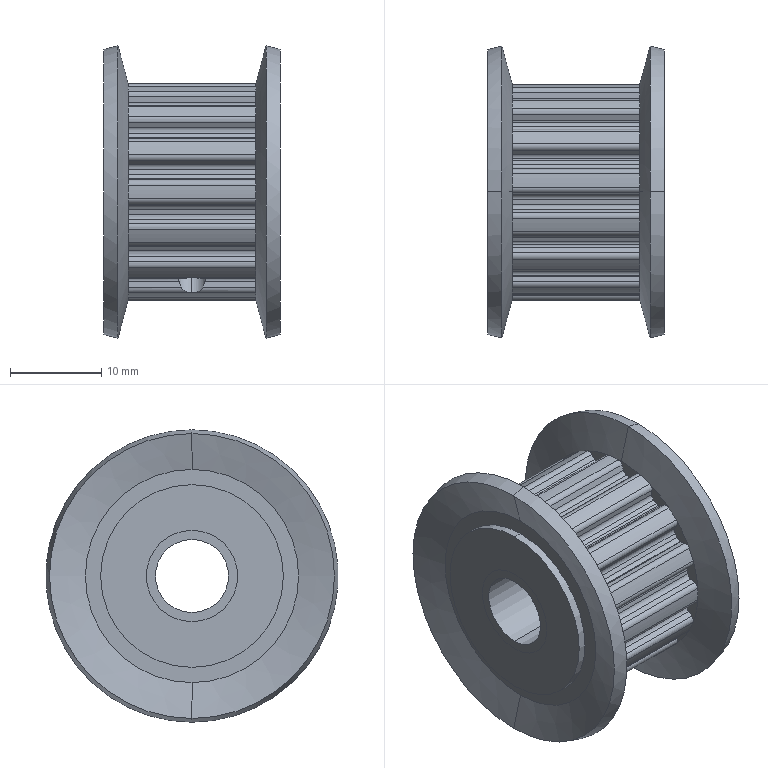Part | NX | features BREP 4 | 4 solids | 248 faces | box 19.302 x 32 x 32 mm | volume 7753 mm3 | cylinder 126 | plane 98 | cone 24 | commonest cylinder face diameters 1.22 x76 20.95 x17 23.75 x15 3.242 x4 4 x4 10 x4